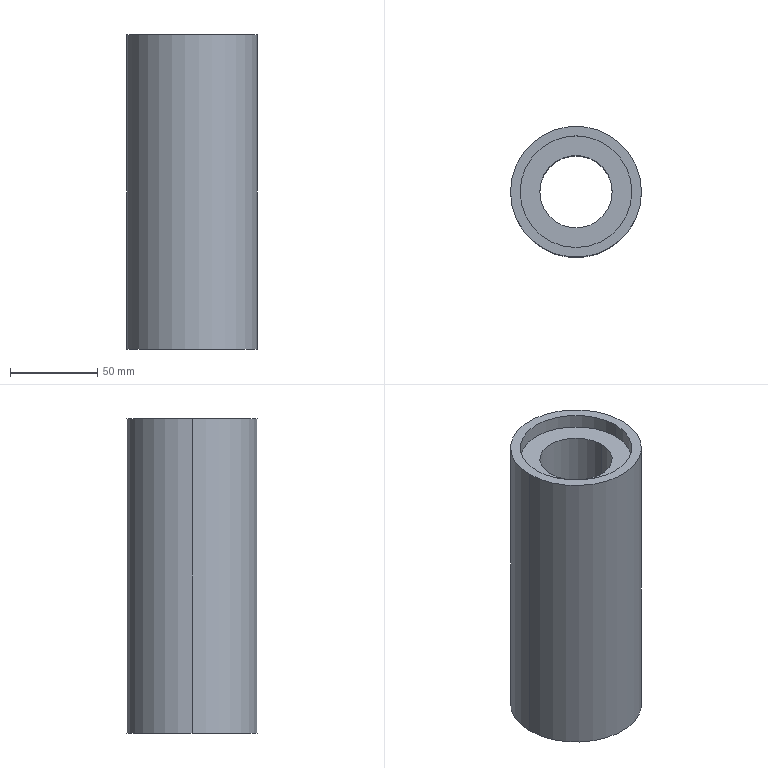Part | STEP file | 1 solid | 12 faces | box 75 x 75 x 180 mm | volume 520275 mm3 | cylinder 8 | plane 4 | commonest cylinder face diameters 41.5 x2 64 x2 66 x2 75 x2
STEP:
#1=CARTESIAN_POINT('',(0.,0.,0.));
#2=DIRECTION('',(0.,0.,1.));
#3=DIRECTION('',(1.,0.,0.));
#4=AXIS2_PLACEMENT_3D('',#1,#2,#3);
#5=CARTESIAN_POINT('',(32.,0.,172.));
#6=VERTEX_POINT('',#5);
#7=CARTESIAN_POINT('',(32.,0.,180.));
#8=VERTEX_POINT('',#7);
#9=CARTESIAN_POINT('',(32.,0.,172.));
#10=DIRECTION('',(0.,0.,1.));
#11=VECTOR('',#10,1.);
#12=LINE('',#9,#11);
#13=CARTESIAN_POINT('',(0.,0.,172.));
#14=DIRECTION('',(0.,0.,1.));
#15=DIRECTION('',(1.,0.,0.));
#16=AXIS2_PLACEMENT_3D('',#13,#14,#15);
#17=CYLINDRICAL_SURFACE('',#16,32.);
#18=CARTESIAN_POINT('',(6.283,0.));
#19=DIRECTION('',(0.,1.));
#20=VECTOR('',#19,1.);
#21=LINE('',#18,#20);
#22=(GEOMETRIC_REPRESENTATION_CONTEXT(2)PARAMETRIC_REPRESENTATION_CONTEXT()REPRESENTATION_CONTEXT('',''));
#23=DEFINITIONAL_REPRESENTATION('',(#21),#22);
#24=PCURVE('',#17,#23);
#25=CARTESIAN_POINT('',(0.,0.,172.));
#26=DIRECTION('',(0.,0.,1.));
#27=DIRECTION('',(1.,0.,0.));
#28=AXIS2_PLACEMENT_3D('',#25,#26,#27);
#29=CYLINDRICAL_SURFACE('',#28,32.);
#30=CARTESIAN_POINT('',(0.,0.));
#31=DIRECTION('',(0.,1.));
#32=VECTOR('',#31,1.);
#33=LINE('',#30,#32);
#34=(GEOMETRIC_REPRESENTATION_CONTEXT(2)PARAMETRIC_REPRESENTATION_CONTEXT()REPRESENTATION_CONTEXT('',''));
#35=DEFINITIONAL_REPRESENTATION('',(#33),#34);
#36=PCURVE('',#29,#35);
#37=SURFACE_CURVE('',#12,(#24,#36),.PCURVE_S1.);
#38=EDGE_CURVE('',#6,#8,#37,.T.);
#39=ORIENTED_EDGE('',*,*,#38,.T.);
#40=CARTESIAN_POINT('',(-32.,0.,180.));
#41=VERTEX_POINT('',#40);
#42=CARTESIAN_POINT('',(0.,0.,180.));
#43=DIRECTION('',(0.,0.,1.));
#44=DIRECTION('',(1.,0.,0.));
#45=AXIS2_PLACEMENT_3D('',#42,#43,#44);
#46=CIRCLE('',#45,32.);
#47=CARTESIAN_POINT('',(0.,8.));
#48=DIRECTION('',(1.,0.));
#49=VECTOR('',#48,1.);
#50=LINE('',#47,#49);
#51=(GEOMETRIC_REPRESENTATION_CONTEXT(2)PARAMETRIC_REPRESENTATION_CONTEXT()REPRESENTATION_CONTEXT('',''));
#52=DEFINITIONAL_REPRESENTATION('',(#50),#51);
#53=PCURVE('',#17,#52);
#54=CARTESIAN_POINT('',(0.,0.,180.));
#55=DIRECTION('',(0.,0.,1.));
#56=DIRECTION('',(1.,0.,0.));
#57=AXIS2_PLACEMENT_3D('',#54,#55,#56);
#58=PLANE('',#57);
#59=CARTESIAN_POINT('',(0.,0.));
#60=DIRECTION('',(1.,0.));
#61=AXIS2_PLACEMENT_2D('',#59,#60);
#62=CIRCLE('',#61,32.);
#63=(GEOMETRIC_REPRESENTATION_CONTEXT(2)PARAMETRIC_REPRESENTATION_CONTEXT()REPRESENTATION_CONTEXT('',''));
#64=DEFINITIONAL_REPRESENTATION('',(#62),#63);
#65=PCURVE('',#58,#64);
#66=SURFACE_CURVE('',#46,(#53,#65),.PCURVE_S1.);
#67=EDGE_CURVE('',#41,#8,#66,.T.);
#68=ORIENTED_EDGE('',*,*,#67,.F.);
#69=CARTESIAN_POINT('',(-32.,0.,172.));
#70=VERTEX_POINT('',#69);
#71=CARTESIAN_POINT('',(-32.,0.,172.));
#72=DIRECTION('',(0.,0.,1.));
#73=VECTOR('',#72,1.);
#74=LINE('',#71,#73);
#75=CARTESIAN_POINT('',(3.142,0.));
#76=DIRECTION('',(0.,1.));
#77=VECTOR('',#76,1.);
#78=LINE('',#75,#77);
#79=(GEOMETRIC_REPRESENTATION_CONTEXT(2)PARAMETRIC_REPRESENTATION_CONTEXT()REPRESENTATION_CONTEXT('',''));
#80=DEFINITIONAL_REPRESENTATION('',(#78),#79);
#81=PCURVE('',#17,#80);
#82=CARTESIAN_POINT('',(3.142,0.));
#83=DIRECTION('',(0.,1.));
#84=VECTOR('',#83,1.);
#85=LINE('',#82,#84);
#86=(GEOMETRIC_REPRESENTATION_CONTEXT(2)PARAMETRIC_REPRESENTATION_CONTEXT()REPRESENTATION_CONTEXT('',''));
#87=DEFINITIONAL_REPRESENTATION('',(#85),#86);
#88=PCURVE('',#29,#87);
#89=SURFACE_CURVE('',#74,(#81,#88),.PCURVE_S1.);
#90=EDGE_CURVE('',#70,#41,#89,.T.);
#91=ORIENTED_EDGE('',*,*,#90,.F.);
#92=CARTESIAN_POINT('',(0.,0.,172.));
#93=DIRECTION('',(0.,0.,1.));
#94=DIRECTION('',(1.,0.,0.));
#95=AXIS2_PLACEMENT_3D('',#92,#93,#94);
#96=CIRCLE('',#95,32.);
#97=CARTESIAN_POINT('',(0.,0.));
#98=DIRECTION('',(1.,0.));
#99=VECTOR('',#98,1.);
#100=LINE('',#97,#99);
#101=(GEOMETRIC_REPRESENTATION_CONTEXT(2)PARAMETRIC_REPRESENTATION_CONTEXT()REPRESENTATION_CONTEXT('',''));
#102=DEFINITIONAL_REPRESENTATION('',(#100),#101);
#103=PCURVE('',#17,#102);
#104=CARTESIAN_POINT('',(0.,0.,172.));
#105=DIRECTION('',(0.,0.,1.));
#106=DIRECTION('',(1.,0.,0.));
#107=AXIS2_PLACEMENT_3D('',#104,#105,#106);
#108=PLANE('',#107);
#109=CARTESIAN_POINT('',(0.,0.));
#110=DIRECTION('',(1.,0.));
#111=AXIS2_PLACEMENT_2D('',#109,#110);
#112=CIRCLE('',#111,32.);
#113=(GEOMETRIC_REPRESENTATION_CONTEXT(2)PARAMETRIC_REPRESENTATION_CONTEXT()REPRESENTATION_CONTEXT('',''));
#114=DEFINITIONAL_REPRESENTATION('',(#112),#113);
#115=PCURVE('',#108,#114);
#116=SURFACE_CURVE('',#96,(#103,#115),.PCURVE_S1.);
#117=EDGE_CURVE('',#70,#6,#116,.T.);
#118=ORIENTED_EDGE('',*,*,#117,.T.);
#119=EDGE_LOOP('',(#39,#68,#91,#118));
#120=FACE_BOUND('',#119,.F.);
#121=ADVANCED_FACE('',(#120),#17,.F.);
#122=CARTESIAN_POINT('',(-33.,0.,8.));
#123=VERTEX_POINT('',#122);
#124=CARTESIAN_POINT('',(-33.,0.,0.));
#125=VERTEX_POINT('',#124);
#126=CARTESIAN_POINT('',(-33.,0.,8.));
#127=DIRECTION('',(0.,0.,-1.));
#128=VECTOR('',#127,1.);
#129=LINE('',#126,#128);
#130=CARTESIAN_POINT('',(0.,0.,8.));
#131=DIRECTION('',(0.,0.,-1.));
#132=DIRECTION('',(-1.,0.,0.));
#133=AXIS2_PLACEMENT_3D('',#130,#131,#132);
#134=CYLINDRICAL_SURFACE('',#133,33.);
#135=CARTESIAN_POINT('',(6.283,0.));
#136=DIRECTION('',(0.,1.));
#137=VECTOR('',#136,1.);
#138=LINE('',#135,#137);
#139=(GEOMETRIC_REPRESENTATION_CONTEXT(2)PARAMETRIC_REPRESENTATION_CONTEXT()REPRESENTATION_CONTEXT('',''));
#140=DEFINITIONAL_REPRESENTATION('',(#138),#139);
#141=PCURVE('',#134,#140);
#142=CARTESIAN_POINT('',(0.,0.,8.));
#143=DIRECTION('',(0.,0.,-1.));
#144=DIRECTION('',(-1.,0.,0.));
#145=AXIS2_PLACEMENT_3D('',#142,#143,#144);
#146=CYLINDRICAL_SURFACE('',#145,33.);
#147=CARTESIAN_POINT('',(0.,0.));
#148=DIRECTION('',(0.,1.));
#149=VECTOR('',#148,1.);
#150=LINE('',#147,#149);
#151=(GEOMETRIC_REPRESENTATION_CONTEXT(2)PARAMETRIC_REPRESENTATION_CONTEXT()REPRESENTATION_CONTEXT('',''));
#152=DEFINITIONAL_REPRESENTATION('',(#150),#151);
#153=PCURVE('',#146,#152);
#154=SURFACE_CURVE('',#129,(#141,#153),.PCURVE_S1.);
#155=EDGE_CURVE('',#123,#125,#154,.T.);
#156=ORIENTED_EDGE('',*,*,#155,.T.);
#157=CARTESIAN_POINT('',(33.,0.,0.));
#158=VERTEX_POINT('',#157);
#159=CARTESIAN_POINT('',(0.,0.,0.));
#160=DIRECTION('',(0.,0.,-1.));
#161=DIRECTION('',(-1.,0.,0.));
#162=AXIS2_PLACEMENT_3D('',#159,#160,#161);
#163=CIRCLE('',#162,33.);
#164=CARTESIAN_POINT('',(0.,8.));
#165=DIRECTION('',(1.,0.));
#166=VECTOR('',#165,1.);
#167=LINE('',#164,#166);
#168=(GEOMETRIC_REPRESENTATION_CONTEXT(2)PARAMETRIC_REPRESENTATION_CONTEXT()REPRESENTATION_CONTEXT('',''));
#169=DEFINITIONAL_REPRESENTATION('',(#167),#168);
#170=PCURVE('',#134,#169);
#171=CARTESIAN_POINT('',(0.,0.,0.));
#172=DIRECTION('',(0.,0.,1.));
#173=DIRECTION('',(1.,0.,0.));
#174=AXIS2_PLACEMENT_3D('',#171,#172,#173);
#175=PLANE('',#174);
#176=CARTESIAN_POINT('',(-33.,0.));
#177=CARTESIAN_POINT('',(-33.,57.158));
#178=CARTESIAN_POINT('',(16.5,28.579));
#179=CARTESIAN_POINT('',(66.,0.));
#180=CARTESIAN_POINT('',(16.5,-28.579));
#181=CARTESIAN_POINT('',(-33.,-57.158));
#182=CARTESIAN_POINT('',(-33.,0.));
#183=(BOUNDED_CURVE()B_SPLINE_CURVE(2,(#176,#177,#178,#179,#180,#181,#182),.UNSPECIFIED.,.T.,.F.)B_SPLINE_CURVE_WITH_KNOTS((1,2,2,2,2,1),(-2.094,0.,2.094,4.189,6.283,8.378),.UNSPECIFIED.)CURVE()GEOMETRIC_REPRESENTATION_ITEM()RATIONAL_B_SPLINE_CURVE((1.,0.5,1.,0.5,1.,0.5,1.))REPRESENTATION_ITEM(''));
#184=(GEOMETRIC_REPRESENTATION_CONTEXT(2)PARAMETRIC_REPRESENTATION_CONTEXT()REPRESENTATION_CONTEXT('',''));
#185=DEFINITIONAL_REPRESENTATION('',(#183),#184);
#186=PCURVE('',#175,#185);
#187=SURFACE_CURVE('',#163,(#170,#186),.PCURVE_S1.);
#188=EDGE_CURVE('',#158,#125,#187,.T.);
#189=ORIENTED_EDGE('',*,*,#188,.F.);
#190=CARTESIAN_POINT('',(33.,0.,8.));
#191=VERTEX_POINT('',#190);
#192=CARTESIAN_POINT('',(33.,0.,8.));
#193=DIRECTION('',(0.,0.,-1.));
#194=VECTOR('',#193,1.);
#195=LINE('',#192,#194);
#196=CARTESIAN_POINT('',(3.142,0.));
#197=DIRECTION('',(0.,1.));
#198=VECTOR('',#197,1.);
#199=LINE('',#196,#198);
#200=(GEOMETRIC_REPRESENTATION_CONTEXT(2)PARAMETRIC_REPRESENTATION_CONTEXT()REPRESENTATION_CONTEXT('',''));
#201=DEFINITIONAL_REPRESENTATION('',(#199),#200);
#202=PCURVE('',#134,#201);
#203=CARTESIAN_POINT('',(3.142,0.));
#204=DIRECTION('',(0.,1.));
#205=VECTOR('',#204,1.);
#206=LINE('',#203,#205);
#207=(GEOMETRIC_REPRESENTATION_CONTEXT(2)PARAMETRIC_REPRESENTATION_CONTEXT()REPRESENTATION_CONTEXT('',''));
#208=DEFINITIONAL_REPRESENTATION('',(#206),#207);
#209=PCURVE('',#146,#208);
#210=SURFACE_CURVE('',#195,(#202,#209),.PCURVE_S1.);
#211=EDGE_CURVE('',#191,#158,#210,.T.);
#212=ORIENTED_EDGE('',*,*,#211,.F.);
#213=CARTESIAN_POINT('',(0.,0.,8.));
#214=DIRECTION('',(0.,0.,-1.));
#215=DIRECTION('',(-1.,0.,0.));
#216=AXIS2_PLACEMENT_3D('',#213,#214,#215);
#217=CIRCLE('',#216,33.);
#218=CARTESIAN_POINT('',(0.,0.));
#219=DIRECTION('',(1.,0.));
#220=VECTOR('',#219,1.);
#221=LINE('',#218,#220);
#222=(GEOMETRIC_REPRESENTATION_CONTEXT(2)PARAMETRIC_REPRESENTATION_CONTEXT()REPRESENTATION_CONTEXT('',''));
#223=DEFINITIONAL_REPRESENTATION('',(#221),#222);
#224=PCURVE('',#134,#223);
#225=CARTESIAN_POINT('',(0.,0.,8.));
#226=DIRECTION('',(0.,0.,-1.));
#227=DIRECTION('',(-1.,0.,0.));
#228=AXIS2_PLACEMENT_3D('',#225,#226,#227);
#229=PLANE('',#228);
#230=CARTESIAN_POINT('',(0.,0.));
#231=DIRECTION('',(1.,0.));
#232=AXIS2_PLACEMENT_2D('',#230,#231);
#233=CIRCLE('',#232,33.);
#234=(GEOMETRIC_REPRESENTATION_CONTEXT(2)PARAMETRIC_REPRESENTATION_CONTEXT()REPRESENTATION_CONTEXT('',''));
#235=DEFINITIONAL_REPRESENTATION('',(#233),#234);
#236=PCURVE('',#229,#235);
#237=SURFACE_CURVE('',#217,(#224,#236),.PCURVE_S1.);
#238=EDGE_CURVE('',#191,#123,#237,.T.);
#239=ORIENTED_EDGE('',*,*,#238,.T.);
#240=EDGE_LOOP('',(#156,#189,#212,#239));
#241=FACE_BOUND('',#240,.F.);
#242=ADVANCED_FACE('',(#241),#134,.F.);
#243=CARTESIAN_POINT('',(37.5,0.,180.));
#244=VERTEX_POINT('',#243);
#245=CARTESIAN_POINT('',(-37.5,0.,180.));
#246=VERTEX_POINT('',#245);
#247=CARTESIAN_POINT('',(0.,0.,180.));
#248=DIRECTION('',(0.,0.,1.));
#249=DIRECTION('',(1.,0.,0.));
#250=AXIS2_PLACEMENT_3D('',#247,#248,#249);
#251=CIRCLE('',#250,37.5);
#252=CARTESIAN_POINT('',(0.,0.,180.));
#253=DIRECTION('',(0.,0.,-1.));
#254=DIRECTION('',(-1.,0.,0.));
#255=AXIS2_PLACEMENT_3D('',#252,#253,#254);
#256=CYLINDRICAL_SURFACE('',#255,37.5);
#257=CARTESIAN_POINT('',(3.142,0.));
#258=DIRECTION('',(-1.,0.));
#259=VECTOR('',#258,1.);
#260=LINE('',#257,#259);
#261=(GEOMETRIC_REPRESENTATION_CONTEXT(2)PARAMETRIC_REPRESENTATION_CONTEXT()REPRESENTATION_CONTEXT('',''));
#262=DEFINITIONAL_REPRESENTATION('',(#260),#261);
#263=PCURVE('',#256,#262);
#264=CARTESIAN_POINT('',(0.,0.));
#265=DIRECTION('',(1.,0.));
#266=AXIS2_PLACEMENT_2D('',#264,#265);
#267=CIRCLE('',#266,37.5);
#268=(GEOMETRIC_REPRESENTATION_CONTEXT(2)PARAMETRIC_REPRESENTATION_CONTEXT()REPRESENTATION_CONTEXT('',''));
#269=DEFINITIONAL_REPRESENTATION('',(#267),#268);
#270=PCURVE('',#58,#269);
#271=SURFACE_CURVE('',#251,(#263,#270),.PCURVE_S1.);
#272=EDGE_CURVE('',#244,#246,#271,.T.);
#273=ORIENTED_EDGE('',*,*,#272,.F.);
#274=CARTESIAN_POINT('',(37.5,0.,0.));
#275=VERTEX_POINT('',#274);
#276=CARTESIAN_POINT('',(37.5,0.,180.));
#277=DIRECTION('',(0.,0.,-1.));
#278=VECTOR('',#277,1.);
#279=LINE('',#276,#278);
#280=CARTESIAN_POINT('',(3.142,0.));
#281=DIRECTION('',(0.,1.));
#282=VECTOR('',#281,1.);
#283=LINE('',#280,#282);
#284=(GEOMETRIC_REPRESENTATION_CONTEXT(2)PARAMETRIC_REPRESENTATION_CONTEXT()REPRESENTATION_CONTEXT('',''));
#285=DEFINITIONAL_REPRESENTATION('',(#283),#284);
#286=PCURVE('',#256,#285);
#287=CARTESIAN_POINT('',(0.,0.,180.));
#288=DIRECTION('',(0.,0.,-1.));
#289=DIRECTION('',(-1.,0.,0.));
#290=AXIS2_PLACEMENT_3D('',#287,#288,#289);
#291=CYLINDRICAL_SURFACE('',#290,37.5);
#292=CARTESIAN_POINT('',(3.142,0.));
#293=DIRECTION('',(0.,1.));
#294=VECTOR('',#293,1.);
#295=LINE('',#292,#294);
#296=(GEOMETRIC_REPRESENTATION_CONTEXT(2)PARAMETRIC_REPRESENTATION_CONTEXT()REPRESENTATION_CONTEXT('',''));
#297=DEFINITIONAL_REPRESENTATION('',(#295),#296);
#298=PCURVE('',#291,#297);
#299=SURFACE_CURVE('',#279,(#286,#298),.PCURVE_S1.);
#300=EDGE_CURVE('',#244,#275,#299,.T.);
#301=ORIENTED_EDGE('',*,*,#300,.T.);
#302=CARTESIAN_POINT('',(-37.5,0.,0.));
#303=VERTEX_POINT('',#302);
#304=CARTESIAN_POINT('',(0.,0.,0.));
#305=DIRECTION('',(0.,0.,1.));
#306=DIRECTION('',(1.,0.,0.));
#307=AXIS2_PLACEMENT_3D('',#304,#305,#306);
#308=CIRCLE('',#307,37.5);
#309=CARTESIAN_POINT('',(3.142,180.));
#310=DIRECTION('',(-1.,0.));
#311=VECTOR('',#310,1.);
#312=LINE('',#309,#311);
#313=(GEOMETRIC_REPRESENTATION_CONTEXT(2)PARAMETRIC_REPRESENTATION_CONTEXT()REPRESENTATION_CONTEXT('',''));
#314=DEFINITIONAL_REPRESENTATION('',(#312),#313);
#315=PCURVE('',#256,#314);
#316=CARTESIAN_POINT('',(0.,0.));
#317=DIRECTION('',(1.,0.));
#318=AXIS2_PLACEMENT_2D('',#316,#317);
#319=CIRCLE('',#318,37.5);
#320=(GEOMETRIC_REPRESENTATION_CONTEXT(2)PARAMETRIC_REPRESENTATION_CONTEXT()REPRESENTATION_CONTEXT('',''));
#321=DEFINITIONAL_REPRESENTATION('',(#319),#320);
#322=PCURVE('',#175,#321);
#323=SURFACE_CURVE('',#308,(#315,#322),.PCURVE_S1.);
#324=EDGE_CURVE('',#275,#303,#323,.T.);
#325=ORIENTED_EDGE('',*,*,#324,.T.);
#326=CARTESIAN_POINT('',(-37.5,0.,180.));
#327=DIRECTION('',(0.,0.,-1.));
#328=VECTOR('',#327,1.);
#329=LINE('',#326,#328);
#330=CARTESIAN_POINT('',(0.,0.));
#331=DIRECTION('',(0.,1.));
#332=VECTOR('',#331,1.);
#333=LINE('',#330,#332);
#334=(GEOMETRIC_REPRESENTATION_CONTEXT(2)PARAMETRIC_REPRESENTATION_CONTEXT()REPRESENTATION_CONTEXT('',''));
#335=DEFINITIONAL_REPRESENTATION('',(#333),#334);
#336=PCURVE('',#256,#335);
#337=CARTESIAN_POINT('',(6.283,0.));
#338=DIRECTION('',(0.,1.));
#339=VECTOR('',#338,1.);
#340=LINE('',#337,#339);
#341=(GEOMETRIC_REPRESENTATION_CONTEXT(2)PARAMETRIC_REPRESENTATION_CONTEXT()REPRESENTATION_CONTEXT('',''));
#342=DEFINITIONAL_REPRESENTATION('',(#340),#341);
#343=PCURVE('',#291,#342);
#344=SURFACE_CURVE('',#329,(#336,#343),.PCURVE_S1.);
#345=EDGE_CURVE('',#246,#303,#344,.T.);
#346=ORIENTED_EDGE('',*,*,#345,.F.);
#347=EDGE_LOOP('',(#273,#301,#325,#346));
#348=FACE_BOUND('',#347,.T.);
#349=ADVANCED_FACE('',(#348),#256,.T.);
#350=CARTESIAN_POINT('',(-20.75,0.,172.));
#351=VERTEX_POINT('',#350);
#352=CARTESIAN_POINT('',(-20.75,0.,8.));
#353=VERTEX_POINT('',#352);
#354=CARTESIAN_POINT('',(-20.75,0.,180.));
#355=DIRECTION('',(0.,0.,-1.));
#356=VECTOR('',#355,1.);
#357=LINE('',#354,#356);
#358=CARTESIAN_POINT('',(0.,0.,180.));
#359=DIRECTION('',(0.,0.,-1.));
#360=DIRECTION('',(-1.,0.,0.));
#361=AXIS2_PLACEMENT_3D('',#358,#359,#360);
#362=CYLINDRICAL_SURFACE('',#361,20.75);
#363=CARTESIAN_POINT('',(6.283,0.));
#364=DIRECTION('',(0.,1.));
#365=VECTOR('',#364,1.);
#366=LINE('',#363,#365);
#367=(GEOMETRIC_REPRESENTATION_CONTEXT(2)PARAMETRIC_REPRESENTATION_CONTEXT()REPRESENTATION_CONTEXT('',''));
#368=DEFINITIONAL_REPRESENTATION('',(#366),#367);
#369=PCURVE('',#362,#368);
#370=CARTESIAN_POINT('',(0.,0.,180.));
#371=DIRECTION('',(0.,0.,-1.));
#372=DIRECTION('',(-1.,0.,0.));
#373=AXIS2_PLACEMENT_3D('',#370,#371,#372);
#374=CYLINDRICAL_SURFACE('',#373,20.75);
#375=CARTESIAN_POINT('',(0.,0.));
#376=DIRECTION('',(0.,1.));
#377=VECTOR('',#376,1.);
#378=LINE('',#375,#377);
#379=(GEOMETRIC_REPRESENTATION_CONTEXT(2)PARAMETRIC_REPRESENTATION_CONTEXT()REPRESENTATION_CONTEXT('',''));
#380=DEFINITIONAL_REPRESENTATION('',(#378),#379);
#381=PCURVE('',#374,#380);
#382=SURFACE_CURVE('',#357,(#369,#381),.PCURVE_S1.);
#383=EDGE_CURVE('',#351,#353,#382,.T.);
#384=ORIENTED_EDGE('',*,*,#383,.T.);
#385=CARTESIAN_POINT('',(20.75,0.,8.));
#386=VERTEX_POINT('',#385);
#387=CARTESIAN_POINT('',(0.,0.,8.));
#388=DIRECTION('',(0.,0.,-1.));
#389=DIRECTION('',(-1.,0.,0.));
#390=AXIS2_PLACEMENT_3D('',#387,#388,#389);
#391=CIRCLE('',#390,20.75);
#392=CARTESIAN_POINT('',(0.,172.));
#393=DIRECTION('',(1.,0.));
#394=VECTOR('',#393,1.);
#395=LINE('',#392,#394);
#396=(GEOMETRIC_REPRESENTATION_CONTEXT(2)PARAMETRIC_REPRESENTATION_CONTEXT()REPRESENTATION_CONTEXT('',''));
#397=DEFINITIONAL_REPRESENTATION('',(#395),#396);
#398=PCURVE('',#362,#397);
#399=CARTESIAN_POINT('',(0.,0.));
#400=DIRECTION('',(1.,0.));
#401=AXIS2_PLACEMENT_2D('',#399,#400);
#402=CIRCLE('',#401,20.75);
#403=(GEOMETRIC_REPRESENTATION_CONTEXT(2)PARAMETRIC_REPRESENTATION_CONTEXT()REPRESENTATION_CONTEXT('',''));
#404=DEFINITIONAL_REPRESENTATION('',(#402),#403);
#405=PCURVE('',#229,#404);
#406=SURFACE_CURVE('',#391,(#398,#405),.PCURVE_S1.);
#407=EDGE_CURVE('',#386,#353,#406,.T.);
#408=ORIENTED_EDGE('',*,*,#407,.F.);
#409=CARTESIAN_POINT('',(20.75,0.,172.));
#410=VERTEX_POINT('',#409);
#411=CARTESIAN_POINT('',(20.75,0.,180.));
#412=DIRECTION('',(0.,0.,-1.));
#413=VECTOR('',#412,1.);
#414=LINE('',#411,#413);
#415=CARTESIAN_POINT('',(3.142,0.));
#416=DIRECTION('',(0.,1.));
#417=VECTOR('',#416,1.);
#418=LINE('',#415,#417);
#419=(GEOMETRIC_REPRESENTATION_CONTEXT(2)PARAMETRIC_REPRESENTATION_CONTEXT()REPRESENTATION_CONTEXT('',''));
#420=DEFINITIONAL_REPRESENTATION('',(#418),#419);
#421=PCURVE('',#362,#420);
#422=CARTESIAN_POINT('',(3.142,0.));
#423=DIRECTION('',(0.,1.));
#424=VECTOR('',#423,1.);
#425=LINE('',#422,#424);
#426=(GEOMETRIC_REPRESENTATION_CONTEXT(2)PARAMETRIC_REPRESENTATION_CONTEXT()REPRESENTATION_CONTEXT('',''));
#427=DEFINITIONAL_REPRESENTATION('',(#425),#426);
#428=PCURVE('',#374,#427);
#429=SURFACE_CURVE('',#414,(#421,#428),.PCURVE_S1.);
#430=EDGE_CURVE('',#410,#386,#429,.T.);
#431=ORIENTED_EDGE('',*,*,#430,.F.);
#432=CARTESIAN_POINT('',(0.,0.,172.));
#433=DIRECTION('',(0.,0.,1.));
#434=DIRECTION('',(1.,0.,0.));
#435=AXIS2_PLACEMENT_3D('',#432,#433,#434);
#436=CIRCLE('',#435,20.75);
#437=CARTESIAN_POINT('',(9.425,8.));
#438=DIRECTION('',(-1.,0.));
#439=VECTOR('',#438,1.);
#440=LINE('',#437,#439);
#441=(GEOMETRIC_REPRESENTATION_CONTEXT(2)PARAMETRIC_REPRESENTATION_CONTEXT()REPRESENTATION_CONTEXT('',''));
#442=DEFINITIONAL_REPRESENTATION('',(#440),#441);
#443=PCURVE('',#362,#442);
#444=CARTESIAN_POINT('',(0.,0.));
#445=DIRECTION('',(1.,0.));
#446=AXIS2_PLACEMENT_2D('',#444,#445);
#447=CIRCLE('',#446,20.75);
#448=(GEOMETRIC_REPRESENTATION_CONTEXT(2)PARAMETRIC_REPRESENTATION_CONTEXT()REPRESENTATION_CONTEXT('',''));
#449=DEFINITIONAL_REPRESENTATION('',(#447),#448);
#450=PCURVE('',#108,#449);
#451=SURFACE_CURVE('',#436,(#443,#450),.PCURVE_S1.);
#452=EDGE_CURVE('',#351,#410,#451,.T.);
#453=ORIENTED_EDGE('',*,*,#452,.F.);
#454=EDGE_LOOP('',(#384,#408,#431,#453));
#455=FACE_BOUND('',#454,.F.);
#456=ADVANCED_FACE('',(#455),#362,.F.);
#457=CARTESIAN_POINT('',(0.,0.,8.));
#458=DIRECTION('',(0.,0.,-1.));
#459=DIRECTION('',(-1.,0.,0.));
#460=AXIS2_PLACEMENT_3D('',#457,#458,#459);
#461=CIRCLE('',#460,20.75);
#462=CARTESIAN_POINT('',(0.,172.));
#463=DIRECTION('',(1.,0.));
#464=VECTOR('',#463,1.);
#465=LINE('',#462,#464);
#466=(GEOMETRIC_REPRESENTATION_CONTEXT(2)PARAMETRIC_REPRESENTATION_CONTEXT()REPRESENTATION_CONTEXT('',''));
#467=DEFINITIONAL_REPRESENTATION('',(#465),#466);
#468=PCURVE('',#374,#467);
#469=CARTESIAN_POINT('',(0.,0.));
#470=DIRECTION('',(1.,0.));
#471=AXIS2_PLACEMENT_2D('',#469,#470);
#472=CIRCLE('',#471,20.75);
#473=(GEOMETRIC_REPRESENTATION_CONTEXT(2)PARAMETRIC_REPRESENTATION_CONTEXT()REPRESENTATION_CONTEXT('',''));
#474=DEFINITIONAL_REPRESENTATION('',(#472),#473);
#475=PCURVE('',#229,#474);
#476=SURFACE_CURVE('',#461,(#468,#475),.PCURVE_S1.);
#477=EDGE_CURVE('',#353,#386,#476,.T.);
#478=ORIENTED_EDGE('',*,*,#477,.F.);
#479=ORIENTED_EDGE('',*,*,#383,.F.);
#480=CARTESIAN_POINT('',(0.,0.,172.));
#481=DIRECTION('',(0.,0.,1.));
#482=DIRECTION('',(1.,0.,0.));
#483=AXIS2_PLACEMENT_3D('',#480,#481,#482);
#484=CIRCLE('',#483,20.75);
#485=CARTESIAN_POINT('',(3.142,8.));
#486=DIRECTION('',(-1.,0.));
#487=VECTOR('',#486,1.);
#488=LINE('',#485,#487);
#489=(GEOMETRIC_REPRESENTATION_CONTEXT(2)PARAMETRIC_REPRESENTATION_CONTEXT()REPRESENTATION_CONTEXT('',''));
#490=DEFINITIONAL_REPRESENTATION('',(#488),#489);
#491=PCURVE('',#374,#490);
#492=CARTESIAN_POINT('',(0.,0.));
#493=DIRECTION('',(1.,0.));
#494=AXIS2_PLACEMENT_2D('',#492,#493);
#495=CIRCLE('',#494,20.75);
#496=(GEOMETRIC_REPRESENTATION_CONTEXT(2)PARAMETRIC_REPRESENTATION_CONTEXT()REPRESENTATION_CONTEXT('',''));
#497=DEFINITIONAL_REPRESENTATION('',(#495),#496);
#498=PCURVE('',#108,#497);
#499=SURFACE_CURVE('',#484,(#491,#498),.PCURVE_S1.);
#500=EDGE_CURVE('',#410,#351,#499,.T.);
#501=ORIENTED_EDGE('',*,*,#500,.F.);
#502=ORIENTED_EDGE('',*,*,#430,.T.);
#503=EDGE_LOOP('',(#478,#479,#501,#502));
#504=FACE_BOUND('',#503,.F.);
#505=ADVANCED_FACE('',(#504),#374,.F.);
#506=CARTESIAN_POINT('',(0.,0.,180.));
#507=DIRECTION('',(0.,0.,1.));
#508=DIRECTION('',(1.,0.,0.));
#509=AXIS2_PLACEMENT_3D('',#506,#507,#508);
#510=CIRCLE('',#509,32.);
#511=CARTESIAN_POINT('',(0.,0.));
#512=DIRECTION('',(1.,0.));
#513=AXIS2_PLACEMENT_2D('',#511,#512);
#514=CIRCLE('',#513,32.);
#515=(GEOMETRIC_REPRESENTATION_CONTEXT(2)PARAMETRIC_REPRESENTATION_CONTEXT()REPRESENTATION_CONTEXT('',''));
#516=DEFINITIONAL_REPRESENTATION('',(#514),#515);
#517=PCURVE('',#58,#516);
#518=CARTESIAN_POINT('',(0.,8.));
#519=DIRECTION('',(1.,0.));
#520=VECTOR('',#519,1.);
#521=LINE('',#518,#520);
#522=(GEOMETRIC_REPRESENTATION_CONTEXT(2)PARAMETRIC_REPRESENTATION_CONTEXT()REPRESENTATION_CONTEXT('',''));
#523=DEFINITIONAL_REPRESENTATION('',(#521),#522);
#524=PCURVE('',#29,#523);
#525=SURFACE_CURVE('',#510,(#517,#524),.PCURVE_S1.);
#526=EDGE_CURVE('',#8,#41,#525,.T.);
#527=ORIENTED_EDGE('',*,*,#526,.F.);
#528=ORIENTED_EDGE('',*,*,#67,.F.);
#529=EDGE_LOOP('',(#527,#528));
#530=FACE_BOUND('',#529,.T.);
#531=CARTESIAN_POINT('',(0.,0.,180.));
#532=DIRECTION('',(0.,0.,1.));
#533=DIRECTION('',(1.,0.,0.));
#534=AXIS2_PLACEMENT_3D('',#531,#532,#533);
#535=CIRCLE('',#534,37.5);
#536=CARTESIAN_POINT('',(0.,0.));
#537=DIRECTION('',(1.,0.));
#538=AXIS2_PLACEMENT_2D('',#536,#537);
#539=CIRCLE('',#538,37.5);
#540=(GEOMETRIC_REPRESENTATION_CONTEXT(2)PARAMETRIC_REPRESENTATION_CONTEXT()REPRESENTATION_CONTEXT('',''));
#541=DEFINITIONAL_REPRESENTATION('',(#539),#540);
#542=PCURVE('',#58,#541);
#543=CARTESIAN_POINT('',(9.425,0.));
#544=DIRECTION('',(-1.,0.));
#545=VECTOR('',#544,1.);
#546=LINE('',#543,#545);
#547=(GEOMETRIC_REPRESENTATION_CONTEXT(2)PARAMETRIC_REPRESENTATION_CONTEXT()REPRESENTATION_CONTEXT('',''));
#548=DEFINITIONAL_REPRESENTATION('',(#546),#547);
#549=PCURVE('',#291,#548);
#550=SURFACE_CURVE('',#535,(#542,#549),.PCURVE_S1.);
#551=EDGE_CURVE('',#246,#244,#550,.T.);
#552=ORIENTED_EDGE('',*,*,#551,.T.);
#553=ORIENTED_EDGE('',*,*,#272,.T.);
#554=EDGE_LOOP('',(#552,#553));
#555=FACE_BOUND('',#554,.T.);
#556=ADVANCED_FACE('',(#530,#555),#58,.T.);
#557=CARTESIAN_POINT('',(0.,0.,0.));
#558=DIRECTION('',(0.,0.,-1.));
#559=DIRECTION('',(-1.,0.,0.));
#560=AXIS2_PLACEMENT_3D('',#557,#558,#559);
#561=CIRCLE('',#560,33.);
#562=CARTESIAN_POINT('',(-33.,0.));
#563=CARTESIAN_POINT('',(-33.,57.158));
#564=CARTESIAN_POINT('',(16.5,28.579));
#565=CARTESIAN_POINT('',(66.,0.));
#566=CARTESIAN_POINT('',(16.5,-28.579));
#567=CARTESIAN_POINT('',(-33.,-57.158));
#568=CARTESIAN_POINT('',(-33.,0.));
#569=(BOUNDED_CURVE()B_SPLINE_CURVE(2,(#562,#563,#564,#565,#566,#567,#568),.UNSPECIFIED.,.T.,.F.)B_SPLINE_CURVE_WITH_KNOTS((1,2,2,2,2,1),(-2.094,0.,2.094,4.189,6.283,8.378),.UNSPECIFIED.)CURVE()GEOMETRIC_REPRESENTATION_ITEM()RATIONAL_B_SPLINE_CURVE((1.,0.5,1.,0.5,1.,0.5,1.))REPRESENTATION_ITEM(''));
#570=(GEOMETRIC_REPRESENTATION_CONTEXT(2)PARAMETRIC_REPRESENTATION_CONTEXT()REPRESENTATION_CONTEXT('',''));
#571=DEFINITIONAL_REPRESENTATION('',(#569),#570);
#572=PCURVE('',#175,#571);
#573=CARTESIAN_POINT('',(0.,8.));
#574=DIRECTION('',(1.,0.));
#575=VECTOR('',#574,1.);
#576=LINE('',#573,#575);
#577=(GEOMETRIC_REPRESENTATION_CONTEXT(2)PARAMETRIC_REPRESENTATION_CONTEXT()REPRESENTATION_CONTEXT('',''));
#578=DEFINITIONAL_REPRESENTATION('',(#576),#577);
#579=PCURVE('',#146,#578);
#580=SURFACE_CURVE('',#561,(#572,#579),.PCURVE_S1.);
#581=EDGE_CURVE('',#125,#158,#580,.T.);
#582=ORIENTED_EDGE('',*,*,#581,.F.);
#583=ORIENTED_EDGE('',*,*,#188,.F.);
#584=EDGE_LOOP('',(#582,#583));
#585=FACE_BOUND('',#584,.T.);
#586=CARTESIAN_POINT('',(0.,0.,0.));
#587=DIRECTION('',(0.,0.,1.));
#588=DIRECTION('',(1.,0.,0.));
#589=AXIS2_PLACEMENT_3D('',#586,#587,#588);
#590=CIRCLE('',#589,37.5);
#591=CARTESIAN_POINT('',(0.,0.));
#592=DIRECTION('',(1.,0.));
#593=AXIS2_PLACEMENT_2D('',#591,#592);
#594=CIRCLE('',#593,37.5);
#595=(GEOMETRIC_REPRESENTATION_CONTEXT(2)PARAMETRIC_REPRESENTATION_CONTEXT()REPRESENTATION_CONTEXT('',''));
#596=DEFINITIONAL_REPRESENTATION('',(#594),#595);
#597=PCURVE('',#175,#596);
#598=CARTESIAN_POINT('',(9.425,180.));
#599=DIRECTION('',(-1.,0.));
#600=VECTOR('',#599,1.);
#601=LINE('',#598,#600);
#602=(GEOMETRIC_REPRESENTATION_CONTEXT(2)PARAMETRIC_REPRESENTATION_CONTEXT()REPRESENTATION_CONTEXT('',''));
#603=DEFINITIONAL_REPRESENTATION('',(#601),#602);
#604=PCURVE('',#291,#603);
#605=SURFACE_CURVE('',#590,(#597,#604),.PCURVE_S1.);
#606=EDGE_CURVE('',#303,#275,#605,.T.);
#607=ORIENTED_EDGE('',*,*,#606,.F.);
#608=ORIENTED_EDGE('',*,*,#324,.F.);
#609=EDGE_LOOP('',(#607,#608));
#610=FACE_BOUND('',#609,.T.);
#611=ADVANCED_FACE('',(#585,#610),#175,.F.);
#612=ORIENTED_EDGE('',*,*,#300,.F.);
#613=ORIENTED_EDGE('',*,*,#551,.F.);
#614=ORIENTED_EDGE('',*,*,#345,.T.);
#615=ORIENTED_EDGE('',*,*,#606,.T.);
#616=EDGE_LOOP('',(#612,#613,#614,#615));
#617=FACE_BOUND('',#616,.T.);
#618=ADVANCED_FACE('',(#617),#291,.T.);
#619=ORIENTED_EDGE('',*,*,#581,.F.);
#620=ORIENTED_EDGE('',*,*,#155,.F.);
#621=CARTESIAN_POINT('',(0.,0.,8.));
#622=DIRECTION('',(0.,0.,-1.));
#623=DIRECTION('',(-1.,0.,0.));
#624=AXIS2_PLACEMENT_3D('',#621,#622,#623);
#625=CIRCLE('',#624,33.);
#626=CARTESIAN_POINT('',(0.,0.));
#627=DIRECTION('',(1.,0.));
#628=VECTOR('',#627,1.);
#629=LINE('',#626,#628);
#630=(GEOMETRIC_REPRESENTATION_CONTEXT(2)PARAMETRIC_REPRESENTATION_CONTEXT()REPRESENTATION_CONTEXT('',''));
#631=DEFINITIONAL_REPRESENTATION('',(#629),#630);
#632=PCURVE('',#146,#631);
#633=CARTESIAN_POINT('',(0.,0.));
#634=DIRECTION('',(1.,0.));
#635=AXIS2_PLACEMENT_2D('',#633,#634);
#636=CIRCLE('',#635,33.);
#637=(GEOMETRIC_REPRESENTATION_CONTEXT(2)PARAMETRIC_REPRESENTATION_CONTEXT()REPRESENTATION_CONTEXT('',''));
#638=DEFINITIONAL_REPRESENTATION('',(#636),#637);
#639=PCURVE('',#229,#638);
#640=SURFACE_CURVE('',#625,(#632,#639),.PCURVE_S1.);
#641=EDGE_CURVE('',#123,#191,#640,.T.);
#642=ORIENTED_EDGE('',*,*,#641,.T.);
#643=ORIENTED_EDGE('',*,*,#211,.T.);
#644=EDGE_LOOP('',(#619,#620,#642,#643));
#645=FACE_BOUND('',#644,.F.);
#646=ADVANCED_FACE('',(#645),#146,.F.);
#647=ORIENTED_EDGE('',*,*,#477,.F.);
#648=ORIENTED_EDGE('',*,*,#407,.F.);
#649=EDGE_LOOP('',(#647,#648));
#650=FACE_BOUND('',#649,.T.);
#651=ORIENTED_EDGE('',*,*,#641,.T.);
#652=ORIENTED_EDGE('',*,*,#238,.T.);
#653=EDGE_LOOP('',(#651,#652));
#654=FACE_BOUND('',#653,.T.);
#655=ADVANCED_FACE('',(#650,#654),#229,.T.);
#656=ORIENTED_EDGE('',*,*,#526,.F.);
#657=ORIENTED_EDGE('',*,*,#38,.F.);
#658=CARTESIAN_POINT('',(0.,0.,172.));
#659=DIRECTION('',(0.,0.,1.));
#660=DIRECTION('',(1.,0.,0.));
#661=AXIS2_PLACEMENT_3D('',#658,#659,#660);
#662=CIRCLE('',#661,32.);
#663=CARTESIAN_POINT('',(0.,0.));
#664=DIRECTION('',(1.,0.));
#665=VECTOR('',#664,1.);
#666=LINE('',#663,#665);
#667=(GEOMETRIC_REPRESENTATION_CONTEXT(2)PARAMETRIC_REPRESENTATION_CONTEXT()REPRESENTATION_CONTEXT('',''));
#668=DEFINITIONAL_REPRESENTATION('',(#666),#667);
#669=PCURVE('',#29,#668);
#670=CARTESIAN_POINT('',(0.,0.));
#671=DIRECTION('',(1.,0.));
#672=AXIS2_PLACEMENT_2D('',#670,#671);
#673=CIRCLE('',#672,32.);
#674=(GEOMETRIC_REPRESENTATION_CONTEXT(2)PARAMETRIC_REPRESENTATION_CONTEXT()REPRESENTATION_CONTEXT('',''));
#675=DEFINITIONAL_REPRESENTATION('',(#673),#674);
#676=PCURVE('',#108,#675);
#677=SURFACE_CURVE('',#662,(#669,#676),.PCURVE_S1.);
#678=EDGE_CURVE('',#6,#70,#677,.T.);
#679=ORIENTED_EDGE('',*,*,#678,.T.);
#680=ORIENTED_EDGE('',*,*,#90,.T.);
#681=EDGE_LOOP('',(#656,#657,#679,#680));
#682=FACE_BOUND('',#681,.F.);
#683=ADVANCED_FACE('',(#682),#29,.F.);
#684=ORIENTED_EDGE('',*,*,#452,.F.);
#685=ORIENTED_EDGE('',*,*,#500,.F.);
#686=EDGE_LOOP('',(#684,#685));
#687=FACE_BOUND('',#686,.T.);
#688=ORIENTED_EDGE('',*,*,#678,.T.);
#689=ORIENTED_EDGE('',*,*,#117,.T.);
#690=EDGE_LOOP('',(#688,#689));
#691=FACE_BOUND('',#690,.T.);
#692=ADVANCED_FACE('',(#687,#691),#108,.T.);
#693=CLOSED_SHELL('',(#121,#242,#349,#456,#505,#556,#611,#618,#646,#655,#683,#692));
#694=MANIFOLD_SOLID_BREP('',#693);
#695=(LENGTH_UNIT()NAMED_UNIT(*)SI_UNIT(.MILLI.,.METRE.));
#696=UNCERTAINTY_MEASURE_WITH_UNIT(LENGTH_MEASURE(0.0000001),#695,'','');
#697=(NAMED_UNIT(*)PLANE_ANGLE_UNIT()SI_UNIT($,.RADIAN.));
#698=(NAMED_UNIT(*)SI_UNIT($,.STERADIAN.)SOLID_ANGLE_UNIT());
#699=(GEOMETRIC_REPRESENTATION_CONTEXT(3)GLOBAL_UNCERTAINTY_ASSIGNED_CONTEXT((#696))GLOBAL_UNIT_ASSIGNED_CONTEXT((#695,#697,#698))REPRESENTATION_CONTEXT('',''));
#700=ADVANCED_BREP_SHAPE_REPRESENTATION('',(#4,#694),#699);